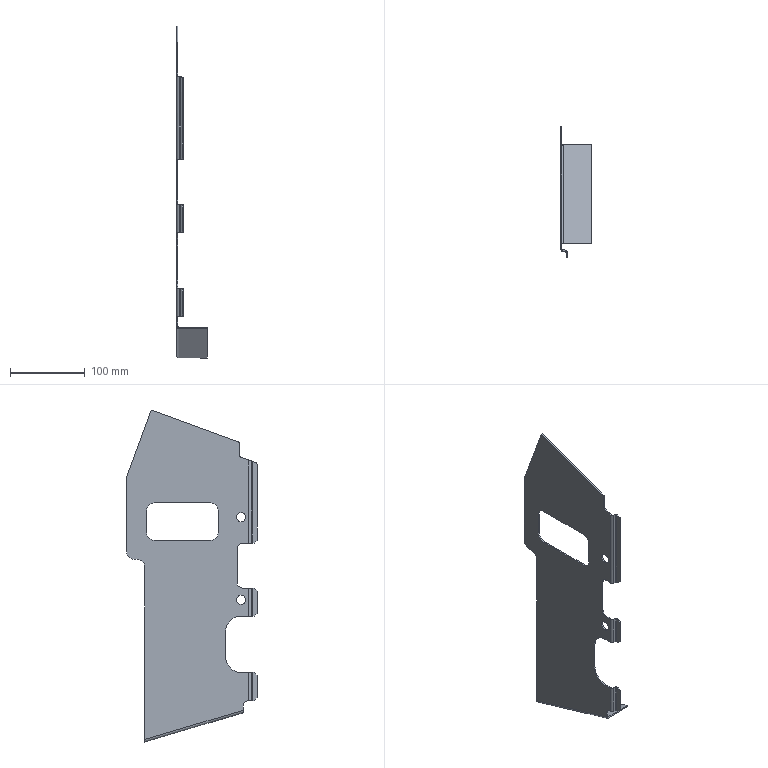Part | SolidWorks | features Fillet 4, EdgeFlange 3, ICE 2, Chamfer 1, FlatPattern 1, SMBaseFlange 1, SheetMetal 1 | 1 solid | 104 faces | box 40.6 x 174 x 442.8 mm | volume 93862 mm3 | plane 68 | cylinder 32 | spline 4 | commonest cylinder face diameters 3.2 x7 6.4 x7 20 x6 12.5 x4 6 x3 14.4 x3